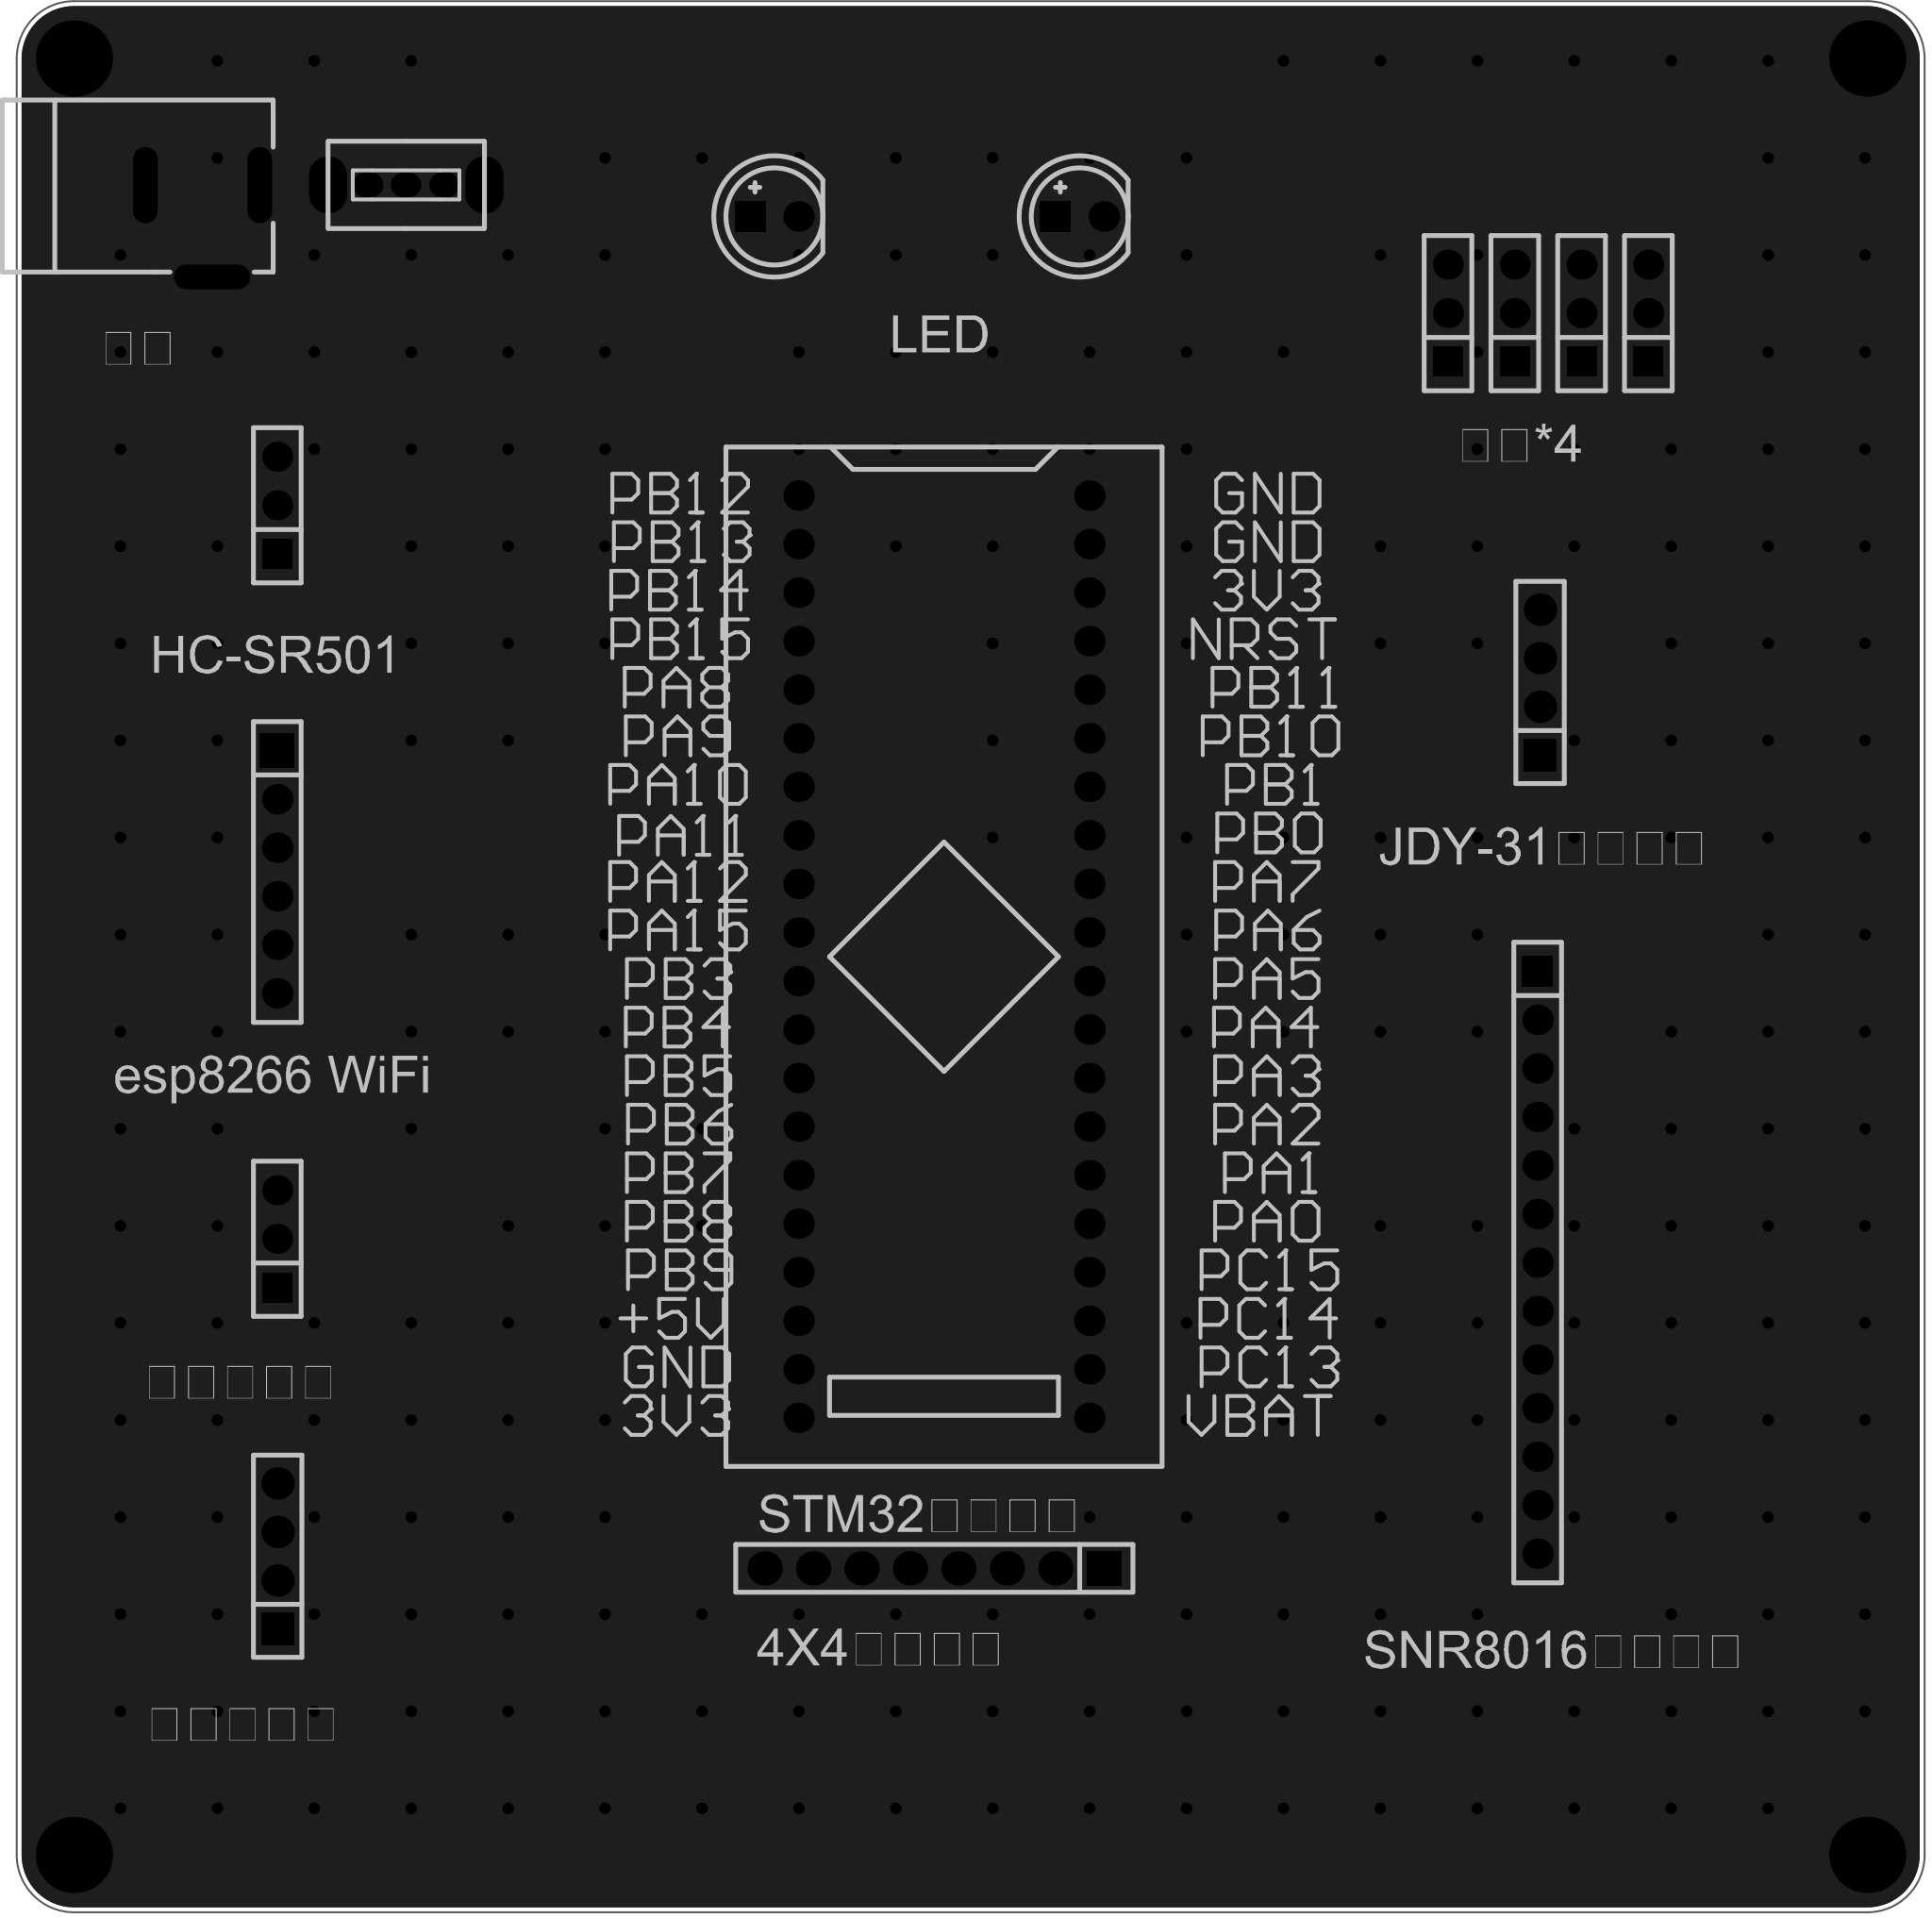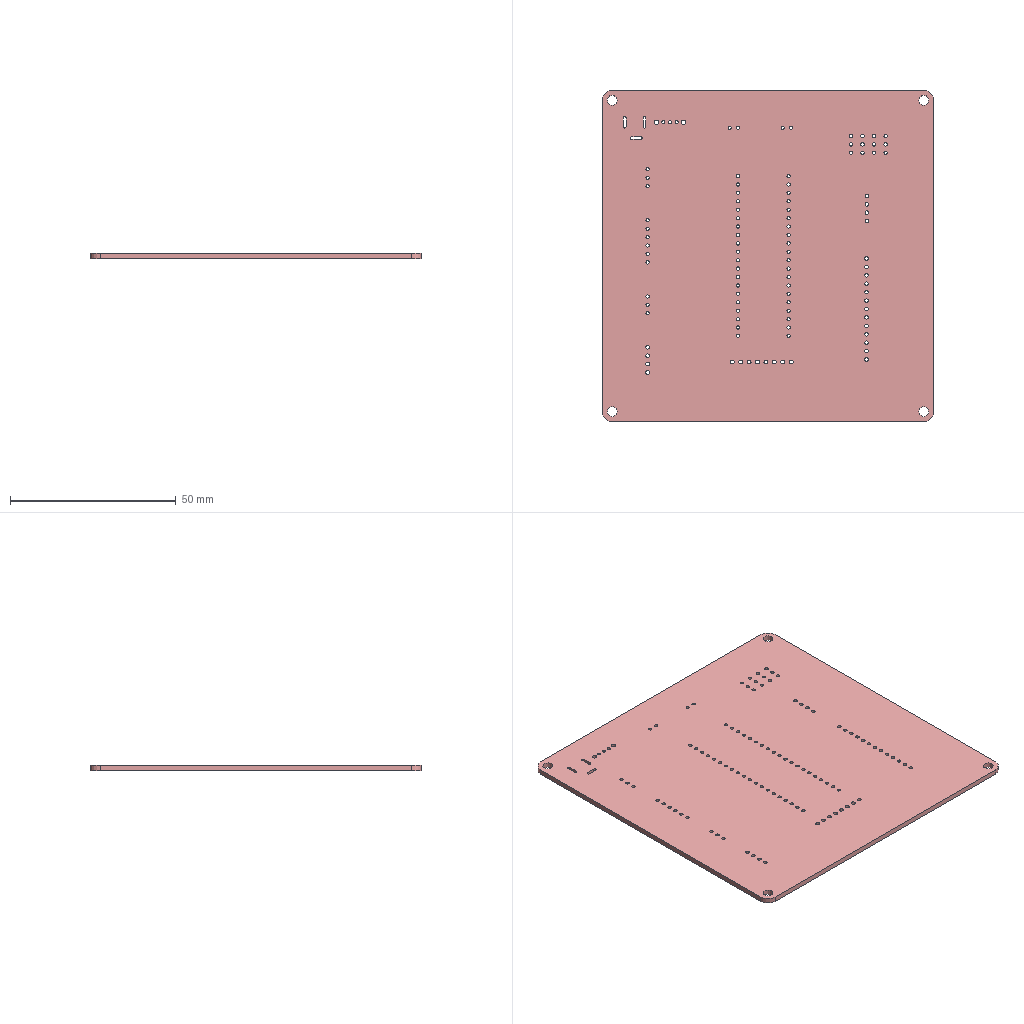Circuit board layout | Altium Designer | box 100 x 100 x 1.6 mm
Layer stack:
# Altium Designer layer stack of  (unit mm; dielectric type: 0 none, 1 core, 2 prepreg, 3 surface material)
index,name,kind,layer,copper_thickness_mm,dielectric_type,dielectric_thickness_mm,dielectric_material,dielectric_constant
0,Top Paste Mask Layer,other,,,,,,
1,Top Silkscreen Layer,other,,,,,,
2,Top Solder Mask Layer,dielectric,,,3,0.01,,3.3
3,Top Layer,copper,Top Layer,0.035,,,,
4,Dielectric1,dielectric,,,3,1.51,FR4,4.5
5,Bottom Layer,copper,Bottom Layer,0.035,,,,
6,Bottom Solder Mask Layer,dielectric,,,3,0.01,,3.3
7,Bottom Silkscreen Layer,other,,,,,,
8,Bottom Paste Mask Layer,other,,,,,,
# drill layer pairs: low layer,high layer
drill_pair,Top Layer,Bottom Layer
Part placement:
Designator,Comment,Layer,Footprint,Center-X(mm),Center-Y(mm),Rotation
U1,STM32F103C8T6-Card,TopLayer,CONN-TH_L53.3-W22.9_STM32F103C8T6-CARD,129.159,128.905,270
H1,,TopLayer,HDR-TH_6P-P2.54-V-F,94.214,133.337,270
H2,,TopLayer,HDR-TH_13P-P2.54-V-F,160.274,112.903,270
H3,,TopLayer,HDR-TH_4P-P2.54-V-F,160.401,143.256,90
H4,,TopLayer,HDR-TH_3P-P2.54-V-F,94.214,152.527,90
H5,,TopLayer,HDR-TH_3P-P2.54-V-F,94.214,114.146,90
H6,,TopLayer,HDR-TH_4P-P2.54-V-F,94.234,97.536,90
H7,,TopLayer,HDR-TH_8P-P2.54-V-F-1,128.651,96.901,180
H8,,TopLayer,HDR-TH_3P-P2.54-V-F,166.077,162.58,90
H9,,TopLayer,HDR-TH_3P-P2.54-V-F,162.577,162.58,90
H10,,TopLayer,HDR-TH_3P-P2.54-V-F,155.575,162.58,90
H11,,TopLayer,HDR-TH_3P-P2.54-V-F,159.076,162.58,90
LED1,,TopLayer,LED-TH_5mm,136.271,167.64,0
LED2,,TopLayer,LED-TH_5mm,120.269,167.64,0
DC1,,TopLayer,DC-2.0,90.297,166.878,180
SW1,,TopLayer,拨动开关,100.973,169.291,0
Pad and via stacks:
# Altium Designer via and pad stacks of  (unit mm). Each distinct definition once, with the count of objects using it.
# via: kind,start_layer,end_layer,hole_mm,diameter_mm,mode(0 simple;1 top-mid-bottom;2 full stack),diameter_per_layer,count,example_net
# pad: kind,layer,hole_mm,hole_type(0 round;1 square;2 slot),plating,top_size,top_shape(1 round;2 rect;3 octagon;9 rounded rect),mid_size,bottom_size,mode,footprint,size_per_layer,count,example
pad,Multi-Layer,3,0,plated,4x4,1,4x4,4x4,0,,,4,1
pad,Multi-Layer,1,0,plated,1.6x1.6,1,1.6x1.6,1.6x1.6,0,CONN-TH_L53.3-W22.9_STM32F103C8T6-CARD,,40,U1.1
pad,Multi-Layer,1.02,0,plated,1.6x1.6,1,1.6x1.6,1.6x1.6,0,HDR-TH_6P-P2.54-V-F,,5,H1.6
pad,Multi-Layer,1.02,0,plated,1.8x1.8,2,1.8x1.8,1.8x1.8,0,HDR-TH_6P-P2.54-V-F,,1,H1.1
pad,Multi-Layer,1.1,0,plated,1.6x1.6,2,1.6x1.6,1.6x1.6,0,HDR-TH_13P-P2.54-V-F,,1,H2.1
pad,Multi-Layer,1.1,0,plated,1.6x1.6,1,1.6x1.6,1.6x1.6,0,HDR-TH_13P-P2.54-V-F,,12,H2.2
pad,Multi-Layer,1.1,0,plated,1.7x1.7,2,1.7x1.7,1.7x1.7,0,HDR-TH_4P-P2.54-V-F,,2,H3.1
pad,Multi-Layer,1.1,0,plated,1.7x1.7,1,1.7x1.7,1.7x1.7,0,HDR-TH_4P-P2.54-V-F,,6,H3.2
pad,Multi-Layer,1.02,0,plated,1.575x1.575,1,1.575x1.575,1.575x1.575,0,HDR-TH_3P-P2.54-V-F,,12,H4.3
pad,Multi-Layer,1.02,0,plated,1.575x1.575,2,1.575x1.575,1.575x1.575,0,HDR-TH_3P-P2.54-V-F,,6,H4.1
pad,Multi-Layer,1.2,0,plated,1.8x1.8,2,1.8x1.8,1.8x1.8,0,HDR-TH_8P-P2.54-V-F-1,,1,H7.1
pad,Multi-Layer,1.2,0,plated,1.8x1.8,1,1.8x1.8,1.8x1.8,0,HDR-TH_8P-P2.54-V-F-1,,7,H7.2
pad,Multi-Layer,1,0,plated,1.6x1.6,2,1.6x1.6,1.6x1.6,0,LED-TH_5mm,,2,LED1.1
pad,Multi-Layer,1,0,plated,1.6x1.6,1,1.6x1.6,1.6x1.6,0,LED-TH_5mm,,2,LED1.2
pad,Multi-Layer,0.8001,2,plated,4x1.3,1,4x1.3,4x1.3,0,DC-2.0,,3,DC1.2
pad,Multi-Layer,0.8992,0,plated,1.6x1.3,1,1.6x1.3,1.6x1.3,0,\u00B2\u00A6\u00B6\u00AF\u00BF\u00AA\u00B9\u00D8,,3,SW1.1
pad,Multi-Layer,1.3,0,plated,3x1.999,1,3x1.999,3x1.999,0,\u00B2\u00A6\u00B6\u00AF\u00BF\u00AA\u00B9\u00D8,,2,SW1.4
via,Top Layer,Bottom Layer,0.3048,0.61,0,,250,GND
Copper pours:
name,layer,net,type(0 solid;1 hatched;2 none)
Bottom Layer-GND,Bottom Layer,GND,0
Top Layer-GND,Top Layer,GND,0
Design rules, without the lines most boards share:
# Altium Designer design rules of  (exported by Altium Designer, unit mm)
# columns: name | kind | enabled | priority | scope1 | scope2 | descriptor | typed fields (field=value)
copperThickness1oz_2 | 2 | enabled | 2 | All | All | Width Constraint (Min=5mil) (Max=100mil) (Preferred=30mil) (All) |
viaSize | 11 | enabled | 1 | All | All | Routing Via (MinHoleWidth=11.811mil) (MaxHoleWidth=248.032mil) (PreferredHoleWidth=12.008mil) (MinWidth=19.685mil) (MaxWidth=393.701mil) (PreferedWidth=24.016mil) (All) | via_min_hole=0.3 via_max_hole=6.3 via_preferred_diameter=0.61 via_preferred_hole=0.305
solderMaskExpansion | 13 | enabled | 2 | All | All | Solder Mask Expansion (Expansion =2.008mil) (All) | expansion=0.051